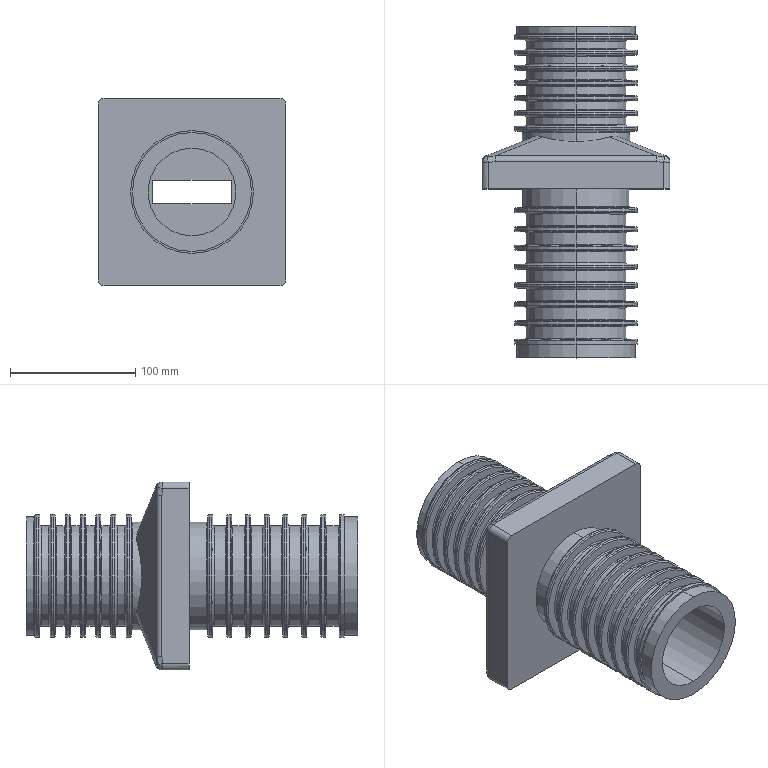Part | STEP file | Through tube 95 | 1 solid | 258 faces | box 150 x 264.782 x 150 mm | volume 1178691 mm3 | torus 116 | cylinder 80 | plane 47 | spline 8 | sphere 7 | commonest cylinder face diameters 98 x30 80 x26 10 x8 40 x4 70 x4 86 x4